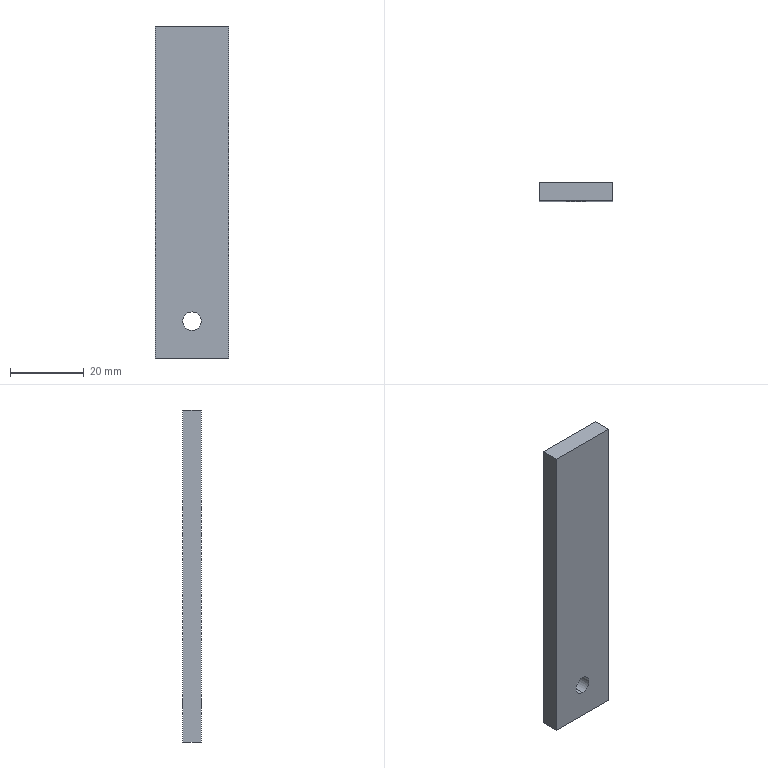Part | SolidWorks | features Extrusion 1 | 1 solid | 8 faces | box 20 x 5 x 90 mm | volume 8902 mm3 | plane 6 | cylinder 2 | commonest cylinder face diameters 5 x2
STEP:
#1=CARTESIAN_POINT('',(0.,5.,-37.5));
#2=VERTEX_POINT('',#1);
#3=CARTESIAN_POINT('',(0.,5.,-32.5));
#4=VERTEX_POINT('',#3);
#5=CARTESIAN_POINT('',(0.,5.,-35.));
#6=DIRECTION('',(0.,1.,0.));
#7=DIRECTION('',(0.,0.,1.));
#8=AXIS2_PLACEMENT_3D('',#5,#6,#7);
#9=CIRCLE('',#8,2.5);
#10=EDGE_CURVE('',#2,#4,#9,.T.);
#11=ORIENTED_EDGE('',*,*,#10,.T.);
#12=CARTESIAN_POINT('',(0.,0.,-32.5));
#13=VERTEX_POINT('',#12);
#14=CARTESIAN_POINT('',(0.,5.,-32.5));
#15=DIRECTION('',(0.,-1.,0.));
#16=VECTOR('',#15,1000.);
#17=LINE('',#14,#16);
#18=EDGE_CURVE('',#4,#13,#17,.T.);
#19=ORIENTED_EDGE('',*,*,#18,.T.);
#20=CARTESIAN_POINT('',(0.,0.,-37.5));
#21=VERTEX_POINT('',#20);
#22=CARTESIAN_POINT('',(0.,0.,-35.));
#23=DIRECTION('',(0.,1.,0.));
#24=DIRECTION('',(0.,0.,1.));
#25=AXIS2_PLACEMENT_3D('',#22,#23,#24);
#26=CIRCLE('',#25,2.5);
#27=EDGE_CURVE('',#21,#13,#26,.T.);
#28=ORIENTED_EDGE('',*,*,#27,.F.);
#29=CARTESIAN_POINT('',(0.,5.,-37.5));
#30=DIRECTION('',(0.,-1.,0.));
#31=VECTOR('',#30,1000.);
#32=LINE('',#29,#31);
#33=EDGE_CURVE('',#2,#21,#32,.T.);
#34=ORIENTED_EDGE('',*,*,#33,.F.);
#35=EDGE_LOOP('',(#11,#19,#28,#34));
#36=FACE_OUTER_BOUND('',#35,.T.);
#37=CARTESIAN_POINT('',(0.,5.,-35.));
#38=DIRECTION('',(0.,-1.,0.));
#39=DIRECTION('',(0.,0.,-1.));
#40=AXIS2_PLACEMENT_3D('',#37,#38,#39);
#41=CYLINDRICAL_SURFACE('',#40,2.5);
#42=ADVANCED_FACE('',(#36),#41,.F.);
#43=CARTESIAN_POINT('',(10.,5.,45.));
#44=VERTEX_POINT('',#43);
#45=CARTESIAN_POINT('',(10.,5.,-45.));
#46=VERTEX_POINT('',#45);
#47=CARTESIAN_POINT('',(10.,5.,45.));
#48=DIRECTION('',(0.,0.,-1.));
#49=VECTOR('',#48,1000.);
#50=LINE('',#47,#49);
#51=EDGE_CURVE('',#44,#46,#50,.T.);
#52=ORIENTED_EDGE('',*,*,#51,.T.);
#53=CARTESIAN_POINT('',(-10.,5.,-45.));
#54=VERTEX_POINT('',#53);
#55=CARTESIAN_POINT('',(-10.,5.,-45.));
#56=DIRECTION('',(-1.,0.,0.));
#57=VECTOR('',#56,1000.);
#58=LINE('',#55,#57);
#59=EDGE_CURVE('',#46,#54,#58,.T.);
#60=ORIENTED_EDGE('',*,*,#59,.T.);
#61=CARTESIAN_POINT('',(-10.,5.,45.));
#62=VERTEX_POINT('',#61);
#63=CARTESIAN_POINT('',(-10.,5.,45.));
#64=DIRECTION('',(0.,0.,1.));
#65=VECTOR('',#64,1000.);
#66=LINE('',#63,#65);
#67=EDGE_CURVE('',#54,#62,#66,.T.);
#68=ORIENTED_EDGE('',*,*,#67,.T.);
#69=CARTESIAN_POINT('',(-10.,5.,45.));
#70=DIRECTION('',(1.,0.,0.));
#71=VECTOR('',#70,1000.);
#72=LINE('',#69,#71);
#73=EDGE_CURVE('',#62,#44,#72,.T.);
#74=ORIENTED_EDGE('',*,*,#73,.T.);
#75=EDGE_LOOP('',(#52,#60,#68,#74));
#76=FACE_OUTER_BOUND('',#75,.T.);
#77=ORIENTED_EDGE('',*,*,#10,.F.);
#78=CARTESIAN_POINT('',(0.,5.,-35.));
#79=DIRECTION('',(0.,1.,0.));
#80=DIRECTION('',(0.,0.,1.));
#81=AXIS2_PLACEMENT_3D('',#78,#79,#80);
#82=CIRCLE('',#81,2.5);
#83=EDGE_CURVE('',#4,#2,#82,.T.);
#84=ORIENTED_EDGE('',*,*,#83,.F.);
#85=EDGE_LOOP('',(#77,#84));
#86=FACE_BOUND('',#85,.T.);
#87=CARTESIAN_POINT('',(0.,5.,0.));
#88=DIRECTION('',(0.,-1.,0.));
#89=DIRECTION('',(0.,0.,-1.));
#90=AXIS2_PLACEMENT_3D('',#87,#88,#89);
#91=PLANE('',#90);
#92=ADVANCED_FACE('',(#76,#86),#91,.F.);
#93=CARTESIAN_POINT('',(10.,0.,45.));
#94=VERTEX_POINT('',#93);
#95=CARTESIAN_POINT('',(10.,0.,-45.));
#96=VERTEX_POINT('',#95);
#97=CARTESIAN_POINT('',(10.,0.,45.));
#98=DIRECTION('',(0.,0.,-1.));
#99=VECTOR('',#98,1000.);
#100=LINE('',#97,#99);
#101=EDGE_CURVE('',#94,#96,#100,.T.);
#102=ORIENTED_EDGE('',*,*,#101,.F.);
#103=CARTESIAN_POINT('',(-10.,0.,45.));
#104=VERTEX_POINT('',#103);
#105=CARTESIAN_POINT('',(-10.,0.,45.));
#106=DIRECTION('',(1.,0.,0.));
#107=VECTOR('',#106,1000.);
#108=LINE('',#105,#107);
#109=EDGE_CURVE('',#104,#94,#108,.T.);
#110=ORIENTED_EDGE('',*,*,#109,.F.);
#111=CARTESIAN_POINT('',(-10.,0.,-45.));
#112=VERTEX_POINT('',#111);
#113=CARTESIAN_POINT('',(-10.,0.,45.));
#114=DIRECTION('',(0.,0.,1.));
#115=VECTOR('',#114,1000.);
#116=LINE('',#113,#115);
#117=EDGE_CURVE('',#112,#104,#116,.T.);
#118=ORIENTED_EDGE('',*,*,#117,.F.);
#119=CARTESIAN_POINT('',(-10.,0.,-45.));
#120=DIRECTION('',(-1.,0.,0.));
#121=VECTOR('',#120,1000.);
#122=LINE('',#119,#121);
#123=EDGE_CURVE('',#96,#112,#122,.T.);
#124=ORIENTED_EDGE('',*,*,#123,.F.);
#125=EDGE_LOOP('',(#102,#110,#118,#124));
#126=FACE_OUTER_BOUND('',#125,.T.);
#127=ORIENTED_EDGE('',*,*,#27,.T.);
#128=CARTESIAN_POINT('',(0.,0.,-35.));
#129=DIRECTION('',(0.,1.,0.));
#130=DIRECTION('',(0.,0.,1.));
#131=AXIS2_PLACEMENT_3D('',#128,#129,#130);
#132=CIRCLE('',#131,2.5);
#133=EDGE_CURVE('',#13,#21,#132,.T.);
#134=ORIENTED_EDGE('',*,*,#133,.T.);
#135=EDGE_LOOP('',(#127,#134));
#136=FACE_BOUND('',#135,.T.);
#137=CARTESIAN_POINT('',(0.,0.,0.));
#138=DIRECTION('',(0.,-1.,0.));
#139=DIRECTION('',(0.,0.,-1.));
#140=AXIS2_PLACEMENT_3D('',#137,#138,#139);
#141=PLANE('',#140);
#142=ADVANCED_FACE('',(#126,#136),#141,.T.);
#143=ORIENTED_EDGE('',*,*,#101,.T.);
#144=CARTESIAN_POINT('',(10.,5.,-45.));
#145=DIRECTION('',(0.,-1.,0.));
#146=VECTOR('',#145,1000.);
#147=LINE('',#144,#146);
#148=EDGE_CURVE('',#46,#96,#147,.T.);
#149=ORIENTED_EDGE('',*,*,#148,.F.);
#150=ORIENTED_EDGE('',*,*,#51,.F.);
#151=CARTESIAN_POINT('',(10.,5.,45.));
#152=DIRECTION('',(0.,-1.,0.));
#153=VECTOR('',#152,1000.);
#154=LINE('',#151,#153);
#155=EDGE_CURVE('',#44,#94,#154,.T.);
#156=ORIENTED_EDGE('',*,*,#155,.T.);
#157=EDGE_LOOP('',(#143,#149,#150,#156));
#158=FACE_OUTER_BOUND('',#157,.T.);
#159=CARTESIAN_POINT('',(10.,5.,45.));
#160=DIRECTION('',(-1.,0.,0.));
#161=DIRECTION('',(0.,0.,1.));
#162=AXIS2_PLACEMENT_3D('',#159,#160,#161);
#163=PLANE('',#162);
#164=ADVANCED_FACE('',(#158),#163,.F.);
#165=ORIENTED_EDGE('',*,*,#123,.T.);
#166=CARTESIAN_POINT('',(-10.,5.,-45.));
#167=DIRECTION('',(0.,-1.,0.));
#168=VECTOR('',#167,1000.);
#169=LINE('',#166,#168);
#170=EDGE_CURVE('',#54,#112,#169,.T.);
#171=ORIENTED_EDGE('',*,*,#170,.F.);
#172=ORIENTED_EDGE('',*,*,#59,.F.);
#173=ORIENTED_EDGE('',*,*,#148,.T.);
#174=EDGE_LOOP('',(#165,#171,#172,#173));
#175=FACE_OUTER_BOUND('',#174,.T.);
#176=CARTESIAN_POINT('',(-10.,5.,-45.));
#177=DIRECTION('',(0.,0.,1.));
#178=DIRECTION('',(1.,0.,0.));
#179=AXIS2_PLACEMENT_3D('',#176,#177,#178);
#180=PLANE('',#179);
#181=ADVANCED_FACE('',(#175),#180,.F.);
#182=ORIENTED_EDGE('',*,*,#117,.T.);
#183=CARTESIAN_POINT('',(-10.,5.,45.));
#184=DIRECTION('',(0.,-1.,0.));
#185=VECTOR('',#184,1000.);
#186=LINE('',#183,#185);
#187=EDGE_CURVE('',#62,#104,#186,.T.);
#188=ORIENTED_EDGE('',*,*,#187,.F.);
#189=ORIENTED_EDGE('',*,*,#67,.F.);
#190=ORIENTED_EDGE('',*,*,#170,.T.);
#191=EDGE_LOOP('',(#182,#188,#189,#190));
#192=FACE_OUTER_BOUND('',#191,.T.);
#193=CARTESIAN_POINT('',(-10.,5.,45.));
#194=DIRECTION('',(1.,0.,0.));
#195=DIRECTION('',(0.,0.,-1.));
#196=AXIS2_PLACEMENT_3D('',#193,#194,#195);
#197=PLANE('',#196);
#198=ADVANCED_FACE('',(#192),#197,.F.);
#199=ORIENTED_EDGE('',*,*,#109,.T.);
#200=ORIENTED_EDGE('',*,*,#155,.F.);
#201=ORIENTED_EDGE('',*,*,#73,.F.);
#202=ORIENTED_EDGE('',*,*,#187,.T.);
#203=EDGE_LOOP('',(#199,#200,#201,#202));
#204=FACE_OUTER_BOUND('',#203,.T.);
#205=CARTESIAN_POINT('',(-10.,5.,45.));
#206=DIRECTION('',(0.,0.,-1.));
#207=DIRECTION('',(-1.,0.,0.));
#208=AXIS2_PLACEMENT_3D('',#205,#206,#207);
#209=PLANE('',#208);
#210=ADVANCED_FACE('',(#204),#209,.F.);
#211=ORIENTED_EDGE('',*,*,#18,.F.);
#212=ORIENTED_EDGE('',*,*,#83,.T.);
#213=ORIENTED_EDGE('',*,*,#33,.T.);
#214=ORIENTED_EDGE('',*,*,#133,.F.);
#215=EDGE_LOOP('',(#211,#212,#213,#214));
#216=FACE_OUTER_BOUND('',#215,.T.);
#217=CARTESIAN_POINT('',(0.,5.,-35.));
#218=DIRECTION('',(0.,-1.,0.));
#219=DIRECTION('',(0.,0.,-1.));
#220=AXIS2_PLACEMENT_3D('',#217,#218,#219);
#221=CYLINDRICAL_SURFACE('',#220,2.5);
#222=ADVANCED_FACE('',(#216),#221,.F.);
#223=CLOSED_SHELL('',(#42,#92,#142,#164,#181,#198,#210,#222));
#224=MANIFOLD_SOLID_BREP('',#223);
#225=CARTESIAN_POINT('',(0.,0.,0.));
#226=DIRECTION('',(0.,0.,1.));
#227=DIRECTION('',(1.,0.,0.));
#228=AXIS2_PLACEMENT_3D('',#225,#226,#227);
#229=(LENGTH_UNIT()NAMED_UNIT(*)SI_UNIT(.MILLI.,.METRE.));
#230=UNCERTAINTY_MEASURE_WITH_UNIT(LENGTH_MEASURE(0.00001),#229,'','');
#231=(NAMED_UNIT(*)PLANE_ANGLE_UNIT()SI_UNIT($,.RADIAN.));
#232=(NAMED_UNIT(*)SI_UNIT($,.STERADIAN.)SOLID_ANGLE_UNIT());
#233=(GEOMETRIC_REPRESENTATION_CONTEXT(3)GLOBAL_UNCERTAINTY_ASSIGNED_CONTEXT((#230))GLOBAL_UNIT_ASSIGNED_CONTEXT((#229,#231,#232))REPRESENTATION_CONTEXT('',''));
#234=ADVANCED_BREP_SHAPE_REPRESENTATION('',(#224,#228),#233);